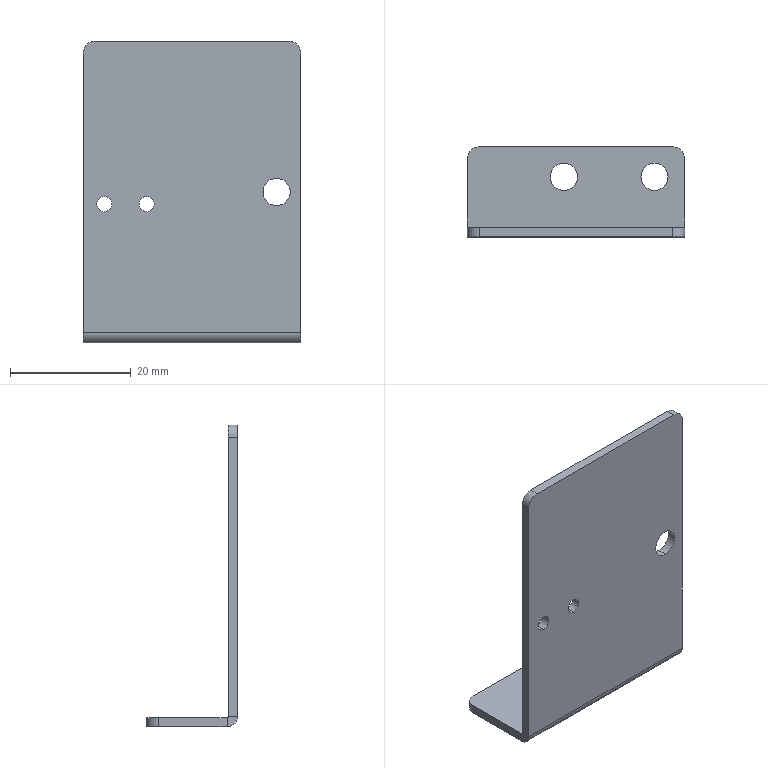Part | STEP file | photoelectric mounting plate | 1 solid | 28 faces | box 36 x 15 x 50 mm | volume 3316 mm3 | cylinder 16 | plane 12 | commonest cylinder face diameters 4.5 x6 2.5 x4 4 x4 0.4 x1 3.4 x1